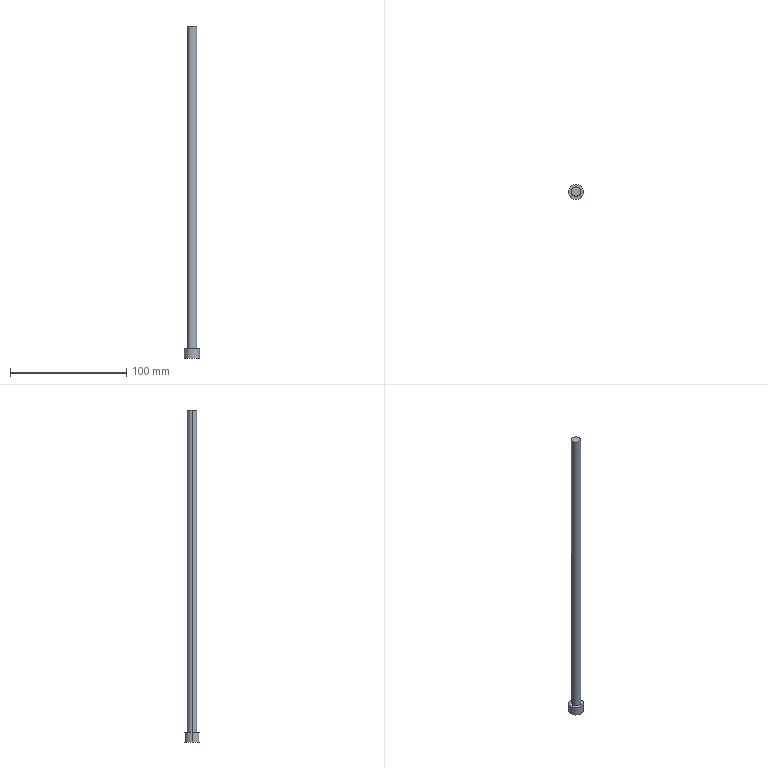Part | Creo | 1 solid | 7 faces | box 13 x 13 x 285.905 mm | volume 15031 mm3 | cylinder 4 | plane 3 | commonest cylinder face diameters 8 x2 13 x2
STEP:
#1=CARTESIAN_POINT('',(4.,35.,25.405));
#2=VERTEX_POINT('',#1);
#3=CARTESIAN_POINT('',(-4.,35.,25.405));
#4=VERTEX_POINT('',#3);
#5=CARTESIAN_POINT('',(0.,35.,25.405));
#6=DIRECTION('',(0.,0.,1.));
#7=DIRECTION('',(1.,0.,0.));
#8=AXIS2_PLACEMENT_3D('',#5,#6,#7);
#9=CIRCLE('',#8,4.);
#10=EDGE_CURVE('',#2,#4,#9,.T.);
#11=ORIENTED_EDGE('',*,*,#10,.F.);
#12=CARTESIAN_POINT('',(0.,35.,25.405));
#13=DIRECTION('',(0.,0.,1.));
#14=DIRECTION('',(-1.,0.,0.));
#15=AXIS2_PLACEMENT_3D('',#12,#13,#14);
#16=CIRCLE('',#15,4.);
#17=EDGE_CURVE('',#4,#2,#16,.T.);
#18=ORIENTED_EDGE('',*,*,#17,.F.);
#19=EDGE_LOOP('',(#11,#18));
#20=FACE_OUTER_BOUND('',#19,.F.);
#21=CARTESIAN_POINT('',(0.,35.,25.405));
#22=DIRECTION('',(0.,0.,1.));
#23=DIRECTION('',(1.,0.,0.));
#24=AXIS2_PLACEMENT_3D('',#21,#22,#23);
#25=PLANE('',#24);
#26=ADVANCED_FACE('',(#20),#25,.T.);
#27=CARTESIAN_POINT('',(-4.,35.,-252.5));
#28=VERTEX_POINT('',#27);
#29=CARTESIAN_POINT('',(4.,35.,-252.5));
#30=VERTEX_POINT('',#29);
#31=CARTESIAN_POINT('',(0.,35.,-252.5));
#32=DIRECTION('',(0.,0.,-1.));
#33=DIRECTION('',(-1.,0.,0.));
#34=AXIS2_PLACEMENT_3D('',#31,#32,#33);
#35=CIRCLE('',#34,4.);
#36=EDGE_CURVE('',#28,#30,#35,.T.);
#37=ORIENTED_EDGE('',*,*,#36,.T.);
#38=CARTESIAN_POINT('',(4.,35.,-252.5));
#39=DIRECTION('',(0.,0.,1.));
#40=VECTOR('',#39,277.905);
#41=LINE('',#38,#40);
#42=EDGE_CURVE('',#30,#2,#41,.T.);
#43=ORIENTED_EDGE('',*,*,#42,.T.);
#44=ORIENTED_EDGE('',*,*,#10,.T.);
#45=CARTESIAN_POINT('',(-4.,35.,-252.5));
#46=DIRECTION('',(0.,0.,1.));
#47=VECTOR('',#46,277.905);
#48=LINE('',#45,#47);
#49=EDGE_CURVE('',#28,#4,#48,.T.);
#50=ORIENTED_EDGE('',*,*,#49,.F.);
#51=EDGE_LOOP('',(#37,#43,#44,#50));
#52=FACE_OUTER_BOUND('',#51,.F.);
#53=CARTESIAN_POINT('',(0.,35.,-255.5));
#54=DIRECTION('',(0.,0.,1.));
#55=DIRECTION('',(1.,0.,0.));
#56=AXIS2_PLACEMENT_3D('',#53,#54,#55);
#57=CYLINDRICAL_SURFACE('',#56,4.);
#58=ADVANCED_FACE('',(#52),#57,.T.);
#59=CARTESIAN_POINT('',(6.5,35.,-252.5));
#60=VERTEX_POINT('',#59);
#61=CARTESIAN_POINT('',(-6.5,35.,-252.5));
#62=VERTEX_POINT('',#61);
#63=CARTESIAN_POINT('',(0.,35.,-252.5));
#64=DIRECTION('',(0.,0.,1.));
#65=DIRECTION('',(1.,0.,0.));
#66=AXIS2_PLACEMENT_3D('',#63,#64,#65);
#67=CIRCLE('',#66,6.5);
#68=EDGE_CURVE('',#60,#62,#67,.T.);
#69=ORIENTED_EDGE('',*,*,#68,.F.);
#70=CARTESIAN_POINT('',(0.,35.,-252.5));
#71=DIRECTION('',(0.,0.,1.));
#72=DIRECTION('',(-1.,0.,0.));
#73=AXIS2_PLACEMENT_3D('',#70,#71,#72);
#74=CIRCLE('',#73,6.5);
#75=EDGE_CURVE('',#62,#60,#74,.T.);
#76=ORIENTED_EDGE('',*,*,#75,.F.);
#77=EDGE_LOOP('',(#69,#76));
#78=FACE_OUTER_BOUND('',#77,.F.);
#79=CARTESIAN_POINT('',(0.,35.,-252.5));
#80=DIRECTION('',(0.,0.,-1.));
#81=DIRECTION('',(1.,0.,0.));
#82=AXIS2_PLACEMENT_3D('',#79,#80,#81);
#83=CIRCLE('',#82,4.);
#84=EDGE_CURVE('',#30,#28,#83,.T.);
#85=ORIENTED_EDGE('',*,*,#84,.F.);
#86=ORIENTED_EDGE('',*,*,#36,.F.);
#87=EDGE_LOOP('',(#85,#86));
#88=FACE_BOUND('',#87,.F.);
#89=CARTESIAN_POINT('',(0.,35.,-252.5));
#90=DIRECTION('',(0.,0.,1.));
#91=DIRECTION('',(1.,0.,0.));
#92=AXIS2_PLACEMENT_3D('',#89,#90,#91);
#93=PLANE('',#92);
#94=ADVANCED_FACE('',(#78,#88),#93,.T.);
#95=ORIENTED_EDGE('',*,*,#84,.T.);
#96=ORIENTED_EDGE('',*,*,#49,.T.);
#97=ORIENTED_EDGE('',*,*,#17,.T.);
#98=ORIENTED_EDGE('',*,*,#42,.F.);
#99=EDGE_LOOP('',(#95,#96,#97,#98));
#100=FACE_OUTER_BOUND('',#99,.F.);
#101=CARTESIAN_POINT('',(0.,35.,-255.5));
#102=DIRECTION('',(0.,0.,1.));
#103=DIRECTION('',(1.,0.,0.));
#104=AXIS2_PLACEMENT_3D('',#101,#102,#103);
#105=CYLINDRICAL_SURFACE('',#104,4.);
#106=ADVANCED_FACE('',(#100),#105,.T.);
#107=ORIENTED_EDGE('',*,*,#68,.T.);
#108=CARTESIAN_POINT('',(-6.5,35.,-260.5));
#109=VERTEX_POINT('',#108);
#110=CARTESIAN_POINT('',(-6.5,35.,-260.5));
#111=DIRECTION('',(0.,0.,1.));
#112=VECTOR('',#111,8.);
#113=LINE('',#110,#112);
#114=EDGE_CURVE('',#109,#62,#113,.T.);
#115=ORIENTED_EDGE('',*,*,#114,.F.);
#116=CARTESIAN_POINT('',(6.5,35.,-260.5));
#117=VERTEX_POINT('',#116);
#118=CARTESIAN_POINT('',(0.,35.,-260.5));
#119=DIRECTION('',(0.,0.,-1.));
#120=DIRECTION('',(-1.,0.,0.));
#121=AXIS2_PLACEMENT_3D('',#118,#119,#120);
#122=CIRCLE('',#121,6.5);
#123=EDGE_CURVE('',#109,#117,#122,.T.);
#124=ORIENTED_EDGE('',*,*,#123,.T.);
#125=CARTESIAN_POINT('',(6.5,35.,-260.5));
#126=DIRECTION('',(0.,0.,1.));
#127=VECTOR('',#126,8.);
#128=LINE('',#125,#127);
#129=EDGE_CURVE('',#117,#60,#128,.T.);
#130=ORIENTED_EDGE('',*,*,#129,.T.);
#131=EDGE_LOOP('',(#107,#115,#124,#130));
#132=FACE_OUTER_BOUND('',#131,.F.);
#133=CARTESIAN_POINT('',(0.,35.,-260.5));
#134=DIRECTION('',(0.,0.,1.));
#135=DIRECTION('',(1.,0.,0.));
#136=AXIS2_PLACEMENT_3D('',#133,#134,#135);
#137=CYLINDRICAL_SURFACE('',#136,6.5);
#138=ADVANCED_FACE('',(#132),#137,.T.);
#139=ORIENTED_EDGE('',*,*,#75,.T.);
#140=ORIENTED_EDGE('',*,*,#129,.F.);
#141=CARTESIAN_POINT('',(0.,35.,-260.5));
#142=DIRECTION('',(0.,0.,-1.));
#143=DIRECTION('',(1.,0.,0.));
#144=AXIS2_PLACEMENT_3D('',#141,#142,#143);
#145=CIRCLE('',#144,6.5);
#146=EDGE_CURVE('',#117,#109,#145,.T.);
#147=ORIENTED_EDGE('',*,*,#146,.T.);
#148=ORIENTED_EDGE('',*,*,#114,.T.);
#149=EDGE_LOOP('',(#139,#140,#147,#148));
#150=FACE_OUTER_BOUND('',#149,.F.);
#151=CARTESIAN_POINT('',(0.,35.,-260.5));
#152=DIRECTION('',(0.,0.,1.));
#153=DIRECTION('',(1.,0.,0.));
#154=AXIS2_PLACEMENT_3D('',#151,#152,#153);
#155=CYLINDRICAL_SURFACE('',#154,6.5);
#156=ADVANCED_FACE('',(#150),#155,.T.);
#157=ORIENTED_EDGE('',*,*,#146,.F.);
#158=ORIENTED_EDGE('',*,*,#123,.F.);
#159=EDGE_LOOP('',(#157,#158));
#160=FACE_OUTER_BOUND('',#159,.F.);
#161=CARTESIAN_POINT('',(0.,35.,-260.5));
#162=DIRECTION('',(0.,0.,-1.));
#163=DIRECTION('',(-1.,0.,0.));
#164=AXIS2_PLACEMENT_3D('',#161,#162,#163);
#165=PLANE('',#164);
#166=ADVANCED_FACE('',(#160),#165,.T.);
#167=CLOSED_SHELL('',(#26,#58,#94,#106,#138,#156,#166));
#168=MANIFOLD_SOLID_BREP('',#167);
#169=(LENGTH_UNIT()NAMED_UNIT(*)SI_UNIT(.MILLI.,.METRE.));
#170=UNCERTAINTY_MEASURE_WITH_UNIT(LENGTH_MEASURE(0.02865),#169,'','');
#171=(NAMED_UNIT(*)PLANE_ANGLE_UNIT()SI_UNIT($,.RADIAN.));
#172=PLANE_ANGLE_MEASURE_WITH_UNIT(PLANE_ANGLE_MEASURE(0.01745),#171);
#173=(CONVERSION_BASED_UNIT('DEGREE',#172)NAMED_UNIT(*)PLANE_ANGLE_UNIT());
#174=(NAMED_UNIT(*)SI_UNIT($,.STERADIAN.)SOLID_ANGLE_UNIT());
#175=(GEOMETRIC_REPRESENTATION_CONTEXT(3)GLOBAL_UNCERTAINTY_ASSIGNED_CONTEXT((#170))GLOBAL_UNIT_ASSIGNED_CONTEXT((#169,#173,#174))REPRESENTATION_CONTEXT('',''));
#176=ADVANCED_BREP_SHAPE_REPRESENTATION('',(#168),#175);